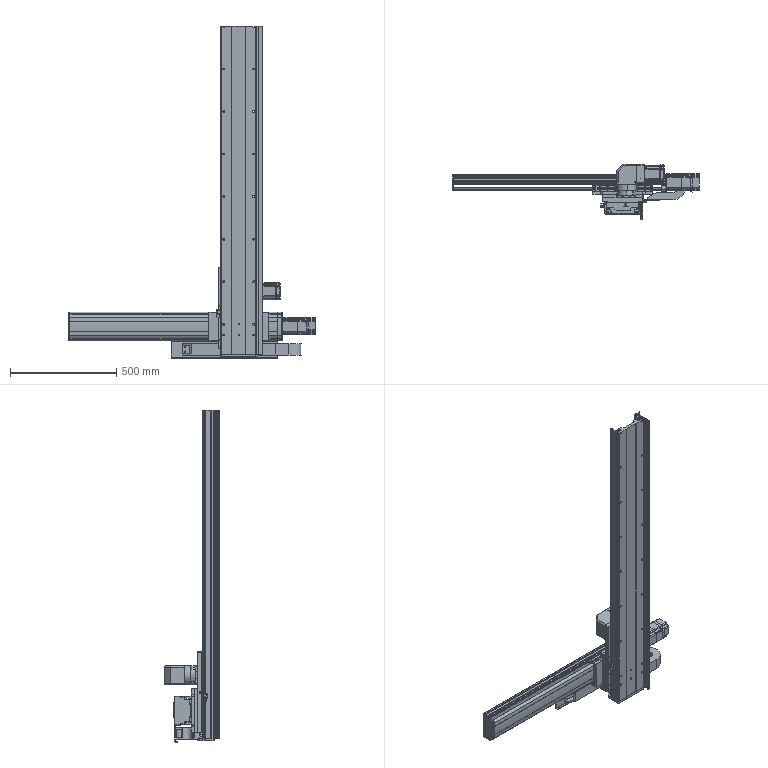Part | STEP file | EH17BEH13-F-3000-600+150BC-W221226YJ01 | 30 solids | 2512 faces | box 1159 x 261.907 x 1561 mm | volume 18211438 mm3 | plane 1189 | cylinder 1093 | cone 182 | spline 32 | torus 16 | commonest cylinder face diameters 1 x83 6 x83 8 x72 5 x58 6.8 x56 8.6 x36